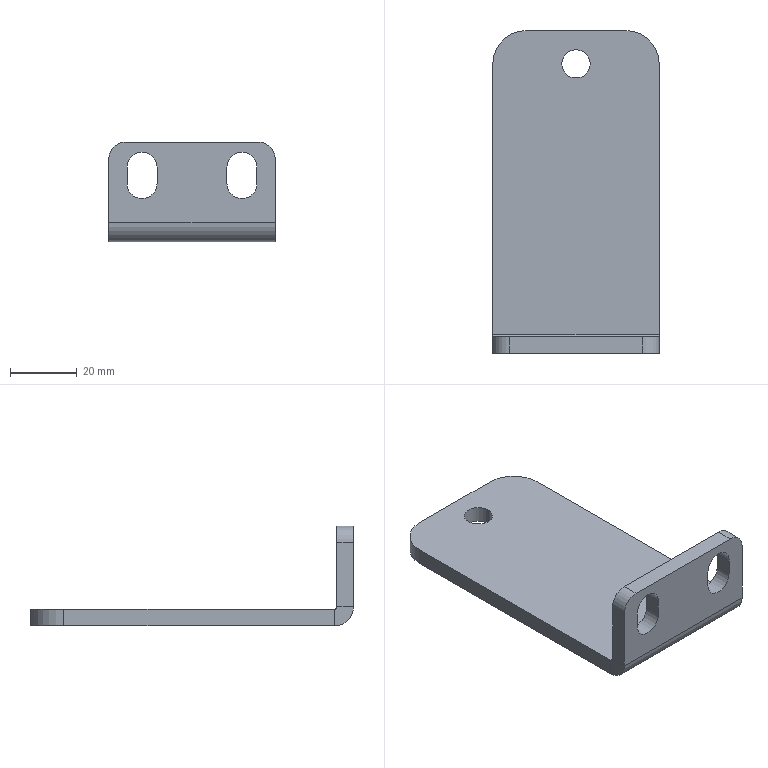Part | SolidWorks | features BaseBody 1 | 1 solid | 30 faces | box 50 x 97 x 30 mm | volume 28515 mm3 | plane 16 | cylinder 14 | commonest cylinder face diameters 9 x6 8.5 x2 10 x2 20 x2 1.473 x1 11.473 x1
STEP:
#1=CARTESIAN_POINT('',(-15.,-48.5,22.));
#2=VERTEX_POINT('',#1);
#3=CARTESIAN_POINT('',(-10.5,-48.5,17.5));
#4=VERTEX_POINT('',#3);
#5=CARTESIAN_POINT('',(-15.,-48.5,17.5));
#6=DIRECTION('',(0.,1.,0.));
#7=DIRECTION('',(0.,0.,1.));
#8=AXIS2_PLACEMENT_3D('',#5,#6,#7);
#9=CIRCLE('',#8,4.5);
#10=EDGE_CURVE('',#2,#4,#9,.T.);
#11=ORIENTED_EDGE('',*,*,#10,.F.);
#12=CARTESIAN_POINT('',(-15.,-43.5,22.));
#13=VERTEX_POINT('',#12);
#14=CARTESIAN_POINT('',(-15.,-53.5,22.));
#15=DIRECTION('',(0.,1.,0.));
#16=VECTOR('',#15,1000.);
#17=LINE('',#14,#16);
#18=EDGE_CURVE('',#2,#13,#17,.T.);
#19=ORIENTED_EDGE('',*,*,#18,.T.);
#20=CARTESIAN_POINT('',(-10.5,-43.5,17.5));
#21=VERTEX_POINT('',#20);
#22=CARTESIAN_POINT('',(-15.,-43.5,17.5));
#23=DIRECTION('',(0.,1.,0.));
#24=DIRECTION('',(0.,0.,1.));
#25=AXIS2_PLACEMENT_3D('',#22,#23,#24);
#26=CIRCLE('',#25,4.5);
#27=EDGE_CURVE('',#13,#21,#26,.T.);
#28=ORIENTED_EDGE('',*,*,#27,.T.);
#29=CARTESIAN_POINT('',(-10.5,-53.5,17.5));
#30=DIRECTION('',(0.,1.,0.));
#31=VECTOR('',#30,1000.);
#32=LINE('',#29,#31);
#33=EDGE_CURVE('',#4,#21,#32,.T.);
#34=ORIENTED_EDGE('',*,*,#33,.F.);
#35=EDGE_LOOP('',(#11,#19,#28,#34));
#36=FACE_OUTER_BOUND('',#35,.T.);
#37=CARTESIAN_POINT('',(-15.,-53.5,17.5));
#38=DIRECTION('',(0.,1.,0.));
#39=DIRECTION('',(0.,0.,1.));
#40=AXIS2_PLACEMENT_3D('',#37,#38,#39);
#41=CYLINDRICAL_SURFACE('',#40,4.5);
#42=ADVANCED_FACE('',(#36),#41,.F.);
#43=CARTESIAN_POINT('',(15.,-48.5,22.));
#44=VERTEX_POINT('',#43);
#45=CARTESIAN_POINT('',(19.5,-48.5,17.5));
#46=VERTEX_POINT('',#45);
#47=CARTESIAN_POINT('',(15.,-48.5,17.5));
#48=DIRECTION('',(0.,1.,0.));
#49=DIRECTION('',(0.,0.,1.));
#50=AXIS2_PLACEMENT_3D('',#47,#48,#49);
#51=CIRCLE('',#50,4.5);
#52=EDGE_CURVE('',#44,#46,#51,.T.);
#53=ORIENTED_EDGE('',*,*,#52,.F.);
#54=CARTESIAN_POINT('',(15.,-43.5,22.));
#55=VERTEX_POINT('',#54);
#56=CARTESIAN_POINT('',(15.,-53.5,22.));
#57=DIRECTION('',(0.,1.,0.));
#58=VECTOR('',#57,1000.);
#59=LINE('',#56,#58);
#60=EDGE_CURVE('',#44,#55,#59,.T.);
#61=ORIENTED_EDGE('',*,*,#60,.T.);
#62=CARTESIAN_POINT('',(19.5,-43.5,17.5));
#63=VERTEX_POINT('',#62);
#64=CARTESIAN_POINT('',(15.,-43.5,17.5));
#65=DIRECTION('',(0.,1.,0.));
#66=DIRECTION('',(0.,0.,1.));
#67=AXIS2_PLACEMENT_3D('',#64,#65,#66);
#68=CIRCLE('',#67,4.5);
#69=EDGE_CURVE('',#55,#63,#68,.T.);
#70=ORIENTED_EDGE('',*,*,#69,.T.);
#71=CARTESIAN_POINT('',(19.5,-53.5,17.5));
#72=DIRECTION('',(0.,1.,0.));
#73=VECTOR('',#72,1000.);
#74=LINE('',#71,#73);
#75=EDGE_CURVE('',#46,#63,#74,.T.);
#76=ORIENTED_EDGE('',*,*,#75,.F.);
#77=EDGE_LOOP('',(#53,#61,#70,#76));
#78=FACE_OUTER_BOUND('',#77,.T.);
#79=CARTESIAN_POINT('',(15.,-53.5,17.5));
#80=DIRECTION('',(0.,1.,0.));
#81=DIRECTION('',(0.,0.,1.));
#82=AXIS2_PLACEMENT_3D('',#79,#80,#81);
#83=CYLINDRICAL_SURFACE('',#82,4.5);
#84=ADVANCED_FACE('',(#78),#83,.F.);
#85=CARTESIAN_POINT('',(-4.25,38.5,-5.));
#86=VERTEX_POINT('',#85);
#87=CARTESIAN_POINT('',(4.25,38.5,-5.));
#88=VERTEX_POINT('',#87);
#89=CARTESIAN_POINT('',(0.,38.5,-5.));
#90=DIRECTION('',(0.,0.,1.));
#91=DIRECTION('',(1.,0.,0.));
#92=AXIS2_PLACEMENT_3D('',#89,#90,#91);
#93=CIRCLE('',#92,4.25);
#94=EDGE_CURVE('',#86,#88,#93,.T.);
#95=ORIENTED_EDGE('',*,*,#94,.F.);
#96=CARTESIAN_POINT('',(-4.25,38.5,0.));
#97=VERTEX_POINT('',#96);
#98=CARTESIAN_POINT('',(-4.25,38.5,-5.));
#99=DIRECTION('',(0.,0.,1.));
#100=VECTOR('',#99,1000.);
#101=LINE('',#98,#100);
#102=EDGE_CURVE('',#86,#97,#101,.T.);
#103=ORIENTED_EDGE('',*,*,#102,.T.);
#104=CARTESIAN_POINT('',(4.25,38.5,0.));
#105=VERTEX_POINT('',#104);
#106=CARTESIAN_POINT('',(0.,38.5,0.));
#107=DIRECTION('',(0.,0.,1.));
#108=DIRECTION('',(1.,0.,0.));
#109=AXIS2_PLACEMENT_3D('',#106,#107,#108);
#110=CIRCLE('',#109,4.25);
#111=EDGE_CURVE('',#97,#105,#110,.T.);
#112=ORIENTED_EDGE('',*,*,#111,.T.);
#113=CARTESIAN_POINT('',(4.25,38.5,-5.));
#114=DIRECTION('',(0.,0.,1.));
#115=VECTOR('',#114,1000.);
#116=LINE('',#113,#115);
#117=EDGE_CURVE('',#88,#105,#116,.T.);
#118=ORIENTED_EDGE('',*,*,#117,.F.);
#119=EDGE_LOOP('',(#95,#103,#112,#118));
#120=FACE_OUTER_BOUND('',#119,.T.);
#121=CARTESIAN_POINT('',(0.,38.5,-5.));
#122=DIRECTION('',(0.,0.,1.));
#123=DIRECTION('',(1.,0.,0.));
#124=AXIS2_PLACEMENT_3D('',#121,#122,#123);
#125=CYLINDRICAL_SURFACE('',#124,4.25);
#126=ADVANCED_FACE('',(#120),#125,.F.);
#127=CARTESIAN_POINT('',(25.,-42.763,0.));
#128=VERTEX_POINT('',#127);
#129=CARTESIAN_POINT('',(25.,38.5,0.));
#130=VERTEX_POINT('',#129);
#131=CARTESIAN_POINT('',(25.,38.5,0.));
#132=DIRECTION('',(0.,1.,0.));
#133=VECTOR('',#132,1000.);
#134=LINE('',#131,#133);
#135=EDGE_CURVE('',#128,#130,#134,.T.);
#136=ORIENTED_EDGE('',*,*,#135,.F.);
#137=CARTESIAN_POINT('',(25.,-42.763,-5.));
#138=VERTEX_POINT('',#137);
#139=CARTESIAN_POINT('',(25.,-42.763,0.));
#140=DIRECTION('',(0.,0.,-1.));
#141=VECTOR('',#140,1000.);
#142=LINE('',#139,#141);
#143=EDGE_CURVE('',#128,#138,#142,.T.);
#144=ORIENTED_EDGE('',*,*,#143,.T.);
#145=CARTESIAN_POINT('',(25.,38.5,-5.));
#146=VERTEX_POINT('',#145);
#147=CARTESIAN_POINT('',(25.,38.5,-5.));
#148=DIRECTION('',(0.,1.,0.));
#149=VECTOR('',#148,1000.);
#150=LINE('',#147,#149);
#151=EDGE_CURVE('',#138,#146,#150,.T.);
#152=ORIENTED_EDGE('',*,*,#151,.T.);
#153=CARTESIAN_POINT('',(25.,38.5,-5.));
#154=DIRECTION('',(0.,0.,1.));
#155=VECTOR('',#154,1000.);
#156=LINE('',#153,#155);
#157=EDGE_CURVE('',#146,#130,#156,.T.);
#158=ORIENTED_EDGE('',*,*,#157,.T.);
#159=EDGE_LOOP('',(#136,#144,#152,#158));
#160=FACE_OUTER_BOUND('',#159,.T.);
#161=CARTESIAN_POINT('',(25.,38.5,-5.));
#162=DIRECTION('',(1.,0.,0.));
#163=DIRECTION('',(0.,1.,0.));
#164=AXIS2_PLACEMENT_3D('',#161,#162,#163);
#165=PLANE('',#164);
#166=ADVANCED_FACE('',(#160),#165,.T.);
#167=CARTESIAN_POINT('',(0.,38.5,-5.));
#168=DIRECTION('',(0.,0.,1.));
#169=DIRECTION('',(1.,0.,0.));
#170=AXIS2_PLACEMENT_3D('',#167,#168,#169);
#171=CIRCLE('',#170,4.25);
#172=EDGE_CURVE('',#88,#86,#171,.T.);
#173=ORIENTED_EDGE('',*,*,#172,.T.);
#174=ORIENTED_EDGE('',*,*,#94,.T.);
#175=EDGE_LOOP('',(#173,#174));
#176=FACE_BOUND('',#175,.T.);
#177=CARTESIAN_POINT('',(-25.,-42.763,-5.));
#178=VERTEX_POINT('',#177);
#179=CARTESIAN_POINT('',(25.,-42.763,-5.));
#180=DIRECTION('',(-1.,0.,0.));
#181=VECTOR('',#180,1000.);
#182=LINE('',#179,#181);
#183=EDGE_CURVE('',#138,#178,#182,.T.);
#184=ORIENTED_EDGE('',*,*,#183,.T.);
#185=CARTESIAN_POINT('',(-25.,38.5,-5.));
#186=VERTEX_POINT('',#185);
#187=CARTESIAN_POINT('',(-25.,38.5,-5.));
#188=DIRECTION('',(0.,-1.,0.));
#189=VECTOR('',#188,1000.);
#190=LINE('',#187,#189);
#191=EDGE_CURVE('',#186,#178,#190,.T.);
#192=ORIENTED_EDGE('',*,*,#191,.F.);
#193=CARTESIAN_POINT('',(-15.,48.5,-5.));
#194=VERTEX_POINT('',#193);
#195=CARTESIAN_POINT('',(-15.,38.5,-5.));
#196=DIRECTION('',(0.,0.,1.));
#197=DIRECTION('',(1.,0.,0.));
#198=AXIS2_PLACEMENT_3D('',#195,#196,#197);
#199=CIRCLE('',#198,10.);
#200=EDGE_CURVE('',#194,#186,#199,.T.);
#201=ORIENTED_EDGE('',*,*,#200,.F.);
#202=CARTESIAN_POINT('',(15.,48.5,-5.));
#203=VERTEX_POINT('',#202);
#204=CARTESIAN_POINT('',(-15.,48.5,-5.));
#205=DIRECTION('',(-1.,0.,0.));
#206=VECTOR('',#205,1000.);
#207=LINE('',#204,#206);
#208=EDGE_CURVE('',#203,#194,#207,.T.);
#209=ORIENTED_EDGE('',*,*,#208,.F.);
#210=CARTESIAN_POINT('',(15.,38.5,-5.));
#211=DIRECTION('',(0.,0.,1.));
#212=DIRECTION('',(-1.,0.,0.));
#213=AXIS2_PLACEMENT_3D('',#210,#211,#212);
#214=CIRCLE('',#213,10.);
#215=EDGE_CURVE('',#146,#203,#214,.T.);
#216=ORIENTED_EDGE('',*,*,#215,.F.);
#217=ORIENTED_EDGE('',*,*,#151,.F.);
#218=EDGE_LOOP('',(#184,#192,#201,#209,#216,#217));
#219=FACE_OUTER_BOUND('',#218,.T.);
#220=CARTESIAN_POINT('',(-15.,38.5,-5.));
#221=DIRECTION('',(0.,0.,1.));
#222=DIRECTION('',(1.,0.,0.));
#223=AXIS2_PLACEMENT_3D('',#220,#221,#222);
#224=PLANE('',#223);
#225=ADVANCED_FACE('',(#176,#219),#224,.F.);
#226=CARTESIAN_POINT('',(0.,38.5,0.));
#227=DIRECTION('',(0.,0.,1.));
#228=DIRECTION('',(1.,0.,0.));
#229=AXIS2_PLACEMENT_3D('',#226,#227,#228);
#230=CIRCLE('',#229,4.25);
#231=EDGE_CURVE('',#105,#97,#230,.T.);
#232=ORIENTED_EDGE('',*,*,#231,.F.);
#233=ORIENTED_EDGE('',*,*,#111,.F.);
#234=EDGE_LOOP('',(#232,#233));
#235=FACE_BOUND('',#234,.T.);
#236=CARTESIAN_POINT('',(-25.,38.5,0.));
#237=VERTEX_POINT('',#236);
#238=CARTESIAN_POINT('',(-25.,-42.763,0.));
#239=VERTEX_POINT('',#238);
#240=CARTESIAN_POINT('',(-25.,38.5,0.));
#241=DIRECTION('',(0.,-1.,0.));
#242=VECTOR('',#241,1000.);
#243=LINE('',#240,#242);
#244=EDGE_CURVE('',#237,#239,#243,.T.);
#245=ORIENTED_EDGE('',*,*,#244,.T.);
#246=CARTESIAN_POINT('',(25.,-42.763,0.));
#247=DIRECTION('',(-1.,0.,0.));
#248=VECTOR('',#247,1000.);
#249=LINE('',#246,#248);
#250=EDGE_CURVE('',#128,#239,#249,.T.);
#251=ORIENTED_EDGE('',*,*,#250,.F.);
#252=ORIENTED_EDGE('',*,*,#135,.T.);
#253=CARTESIAN_POINT('',(15.,48.5,0.));
#254=VERTEX_POINT('',#253);
#255=CARTESIAN_POINT('',(15.,38.5,0.));
#256=DIRECTION('',(0.,0.,1.));
#257=DIRECTION('',(-1.,0.,0.));
#258=AXIS2_PLACEMENT_3D('',#255,#256,#257);
#259=CIRCLE('',#258,10.);
#260=EDGE_CURVE('',#130,#254,#259,.T.);
#261=ORIENTED_EDGE('',*,*,#260,.T.);
#262=CARTESIAN_POINT('',(-15.,48.5,0.));
#263=VERTEX_POINT('',#262);
#264=CARTESIAN_POINT('',(-15.,48.5,0.));
#265=DIRECTION('',(-1.,0.,0.));
#266=VECTOR('',#265,1000.);
#267=LINE('',#264,#266);
#268=EDGE_CURVE('',#254,#263,#267,.T.);
#269=ORIENTED_EDGE('',*,*,#268,.T.);
#270=CARTESIAN_POINT('',(-15.,38.5,0.));
#271=DIRECTION('',(0.,0.,1.));
#272=DIRECTION('',(1.,0.,0.));
#273=AXIS2_PLACEMENT_3D('',#270,#271,#272);
#274=CIRCLE('',#273,10.);
#275=EDGE_CURVE('',#263,#237,#274,.T.);
#276=ORIENTED_EDGE('',*,*,#275,.T.);
#277=EDGE_LOOP('',(#245,#251,#252,#261,#269,#276));
#278=FACE_OUTER_BOUND('',#277,.T.);
#279=CARTESIAN_POINT('',(-15.,38.5,0.));
#280=DIRECTION('',(0.,0.,1.));
#281=DIRECTION('',(1.,0.,0.));
#282=AXIS2_PLACEMENT_3D('',#279,#280,#281);
#283=PLANE('',#282);
#284=ADVANCED_FACE('',(#235,#278),#283,.T.);
#285=CARTESIAN_POINT('',(-25.,-42.763,0.));
#286=DIRECTION('',(0.,0.,-1.));
#287=VECTOR('',#286,1000.);
#288=LINE('',#285,#287);
#289=EDGE_CURVE('',#239,#178,#288,.T.);
#290=ORIENTED_EDGE('',*,*,#289,.F.);
#291=ORIENTED_EDGE('',*,*,#244,.F.);
#292=CARTESIAN_POINT('',(-25.,38.5,-5.));
#293=DIRECTION('',(0.,0.,1.));
#294=VECTOR('',#293,1000.);
#295=LINE('',#292,#294);
#296=EDGE_CURVE('',#186,#237,#295,.T.);
#297=ORIENTED_EDGE('',*,*,#296,.F.);
#298=ORIENTED_EDGE('',*,*,#191,.T.);
#299=EDGE_LOOP('',(#290,#291,#297,#298));
#300=FACE_OUTER_BOUND('',#299,.T.);
#301=CARTESIAN_POINT('',(-25.,38.5,-5.));
#302=DIRECTION('',(-1.,0.,0.));
#303=DIRECTION('',(0.,-1.,0.));
#304=AXIS2_PLACEMENT_3D('',#301,#302,#303);
#305=PLANE('',#304);
#306=ADVANCED_FACE('',(#300),#305,.T.);
#307=ORIENTED_EDGE('',*,*,#275,.F.);
#308=CARTESIAN_POINT('',(-15.,48.5,-5.));
#309=DIRECTION('',(0.,0.,1.));
#310=VECTOR('',#309,1000.);
#311=LINE('',#308,#310);
#312=EDGE_CURVE('',#194,#263,#311,.T.);
#313=ORIENTED_EDGE('',*,*,#312,.F.);
#314=ORIENTED_EDGE('',*,*,#200,.T.);
#315=ORIENTED_EDGE('',*,*,#296,.T.);
#316=EDGE_LOOP('',(#307,#313,#314,#315));
#317=FACE_OUTER_BOUND('',#316,.T.);
#318=CARTESIAN_POINT('',(-15.,38.5,-5.));
#319=DIRECTION('',(0.,0.,1.));
#320=DIRECTION('',(1.,0.,0.));
#321=AXIS2_PLACEMENT_3D('',#318,#319,#320);
#322=CYLINDRICAL_SURFACE('',#321,10.);
#323=ADVANCED_FACE('',(#317),#322,.T.);
#324=ORIENTED_EDGE('',*,*,#268,.F.);
#325=CARTESIAN_POINT('',(15.,48.5,-5.));
#326=DIRECTION('',(0.,0.,1.));
#327=VECTOR('',#326,1000.);
#328=LINE('',#325,#327);
#329=EDGE_CURVE('',#203,#254,#328,.T.);
#330=ORIENTED_EDGE('',*,*,#329,.F.);
#331=ORIENTED_EDGE('',*,*,#208,.T.);
#332=ORIENTED_EDGE('',*,*,#312,.T.);
#333=EDGE_LOOP('',(#324,#330,#331,#332));
#334=FACE_OUTER_BOUND('',#333,.T.);
#335=CARTESIAN_POINT('',(-15.,48.5,-5.));
#336=DIRECTION('',(0.,1.,0.));
#337=DIRECTION('',(0.,0.,1.));
#338=AXIS2_PLACEMENT_3D('',#335,#336,#337);
#339=PLANE('',#338);
#340=ADVANCED_FACE('',(#334),#339,.T.);
#341=ORIENTED_EDGE('',*,*,#260,.F.);
#342=ORIENTED_EDGE('',*,*,#157,.F.);
#343=ORIENTED_EDGE('',*,*,#215,.T.);
#344=ORIENTED_EDGE('',*,*,#329,.T.);
#345=EDGE_LOOP('',(#341,#342,#343,#344));
#346=FACE_OUTER_BOUND('',#345,.T.);
#347=CARTESIAN_POINT('',(15.,38.5,-5.));
#348=DIRECTION('',(0.,0.,1.));
#349=DIRECTION('',(1.,0.,0.));
#350=AXIS2_PLACEMENT_3D('',#347,#348,#349);
#351=CYLINDRICAL_SURFACE('',#350,10.);
#352=ADVANCED_FACE('',(#346),#351,.T.);
#353=ORIENTED_EDGE('',*,*,#102,.F.);
#354=ORIENTED_EDGE('',*,*,#172,.F.);
#355=ORIENTED_EDGE('',*,*,#117,.T.);
#356=ORIENTED_EDGE('',*,*,#231,.T.);
#357=EDGE_LOOP('',(#353,#354,#355,#356));
#358=FACE_OUTER_BOUND('',#357,.T.);
#359=CARTESIAN_POINT('',(0.,38.5,-5.));
#360=DIRECTION('',(0.,0.,1.));
#361=DIRECTION('',(1.,0.,0.));
#362=AXIS2_PLACEMENT_3D('',#359,#360,#361);
#363=CYLINDRICAL_SURFACE('',#362,4.25);
#364=ADVANCED_FACE('',(#358),#363,.F.);
#365=CARTESIAN_POINT('',(-25.,-43.5,0.7366));
#366=VERTEX_POINT('',#365);
#367=CARTESIAN_POINT('',(-25.,-48.5,0.7366));
#368=VERTEX_POINT('',#367);
#369=CARTESIAN_POINT('',(-25.,-48.5,0.7366));
#370=DIRECTION('',(0.,-1.,0.));
#371=VECTOR('',#370,1000.);
#372=LINE('',#369,#371);
#373=EDGE_CURVE('',#366,#368,#372,.T.);
#374=ORIENTED_EDGE('',*,*,#373,.F.);
#375=CARTESIAN_POINT('',(-25.,-42.763,0.7366));
#376=DIRECTION('',(-1.,0.,0.));
#377=DIRECTION('',(0.,0.,-1.));
#378=AXIS2_PLACEMENT_3D('',#375,#376,#377);
#379=CIRCLE('',#378,0.7366);
#380=EDGE_CURVE('',#239,#366,#379,.T.);
#381=ORIENTED_EDGE('',*,*,#380,.F.);
#382=ORIENTED_EDGE('',*,*,#289,.T.);
#383=CARTESIAN_POINT('',(-25.,-42.763,0.7366));
#384=DIRECTION('',(-1.,0.,0.));
#385=DIRECTION('',(0.,0.,-1.));
#386=AXIS2_PLACEMENT_3D('',#383,#384,#385);
#387=CIRCLE('',#386,5.737);
#388=EDGE_CURVE('',#178,#368,#387,.T.);
#389=ORIENTED_EDGE('',*,*,#388,.T.);
#390=EDGE_LOOP('',(#374,#381,#382,#389));
#391=FACE_OUTER_BOUND('',#390,.T.);
#392=CARTESIAN_POINT('',(-25.,-42.763,0.7366));
#393=DIRECTION('',(-1.,0.,0.));
#394=DIRECTION('',(0.,0.,1.));
#395=AXIS2_PLACEMENT_3D('',#392,#393,#394);
#396=PLANE('',#395);
#397=ADVANCED_FACE('',(#391),#396,.T.);
#398=CARTESIAN_POINT('',(25.,-43.5,0.7366));
#399=VERTEX_POINT('',#398);
#400=CARTESIAN_POINT('',(25.,-42.763,0.7366));
#401=DIRECTION('',(1.,0.,0.));
#402=DIRECTION('',(0.,0.,-1.));
#403=AXIS2_PLACEMENT_3D('',#400,#401,#402);
#404=CIRCLE('',#403,0.7366);
#405=EDGE_CURVE('',#399,#128,#404,.T.);
#406=ORIENTED_EDGE('',*,*,#405,.F.);
#407=CARTESIAN_POINT('',(25.,-48.5,0.7366));
#408=VERTEX_POINT('',#407);
#409=CARTESIAN_POINT('',(25.,-43.5,0.7366));
#410=DIRECTION('',(0.,-1.,0.));
#411=VECTOR('',#410,1000.);
#412=LINE('',#409,#411);
#413=EDGE_CURVE('',#399,#408,#412,.T.);
#414=ORIENTED_EDGE('',*,*,#413,.T.);
#415=CARTESIAN_POINT('',(25.,-42.763,0.7366));
#416=DIRECTION('',(1.,0.,0.));
#417=DIRECTION('',(0.,0.,-1.));
#418=AXIS2_PLACEMENT_3D('',#415,#416,#417);
#419=CIRCLE('',#418,5.737);
#420=EDGE_CURVE('',#408,#138,#419,.T.);
#421=ORIENTED_EDGE('',*,*,#420,.T.);
#422=ORIENTED_EDGE('',*,*,#143,.F.);
#423=EDGE_LOOP('',(#406,#414,#421,#422));
#424=FACE_OUTER_BOUND('',#423,.T.);
#425=CARTESIAN_POINT('',(25.,-42.763,0.7366));
#426=DIRECTION('',(-1.,0.,0.));
#427=DIRECTION('',(0.,0.,1.));
#428=AXIS2_PLACEMENT_3D('',#425,#426,#427);
#429=PLANE('',#428);
#430=ADVANCED_FACE('',(#424),#429,.F.);
#431=ORIENTED_EDGE('',*,*,#183,.F.);
#432=ORIENTED_EDGE('',*,*,#420,.F.);
#433=CARTESIAN_POINT('',(-25.,-48.5,0.7366));
#434=DIRECTION('',(-1.,0.,0.));
#435=VECTOR('',#434,1000.);
#436=LINE('',#433,#435);
#437=EDGE_CURVE('',#408,#368,#436,.T.);
#438=ORIENTED_EDGE('',*,*,#437,.T.);
#439=ORIENTED_EDGE('',*,*,#388,.F.);
#440=EDGE_LOOP('',(#431,#432,#438,#439));
#441=FACE_OUTER_BOUND('',#440,.T.);
#442=CARTESIAN_POINT('',(25.,-42.763,0.7366));
#443=DIRECTION('',(1.,0.,0.));
#444=DIRECTION('',(0.,-1.,0.));
#445=AXIS2_PLACEMENT_3D('',#442,#443,#444);
#446=CYLINDRICAL_SURFACE('',#445,5.737);
#447=ADVANCED_FACE('',(#441),#446,.T.);
#448=ORIENTED_EDGE('',*,*,#250,.T.);
#449=ORIENTED_EDGE('',*,*,#380,.T.);
#450=CARTESIAN_POINT('',(-25.,-43.5,0.7366));
#451=DIRECTION('',(1.,0.,0.));
#452=VECTOR('',#451,1000.);
#453=LINE('',#450,#452);
#454=EDGE_CURVE('',#366,#399,#453,.T.);
#455=ORIENTED_EDGE('',*,*,#454,.T.);
#456=ORIENTED_EDGE('',*,*,#405,.T.);
#457=EDGE_LOOP('',(#448,#449,#455,#456));
#458=FACE_OUTER_BOUND('',#457,.T.);
#459=CARTESIAN_POINT('',(25.,-42.763,0.7366));
#460=DIRECTION('',(1.,0.,0.));
#461=DIRECTION('',(0.,-1.,0.));
#462=AXIS2_PLACEMENT_3D('',#459,#460,#461);
#463=CYLINDRICAL_SURFACE('',#462,0.7366);
#464=ADVANCED_FACE('',(#458),#463,.F.);
#465=CARTESIAN_POINT('',(-25.,-48.5,20.));
#466=VERTEX_POINT('',#465);
#467=CARTESIAN_POINT('',(-25.,-48.5,0.));
#468=DIRECTION('',(0.,0.,-1.));
#469=VECTOR('',#468,1000.);
#470=LINE('',#467,#469);
#471=EDGE_CURVE('',#466,#368,#470,.T.);
#472=ORIENTED_EDGE('',*,*,#471,.F.);
#473=CARTESIAN_POINT('',(-25.,-43.5,20.));
#474=VERTEX_POINT('',#473);
#475=CARTESIAN_POINT('',(-25.,-48.5,20.));
#476=DIRECTION('',(0.,1.,0.));
#477=VECTOR('',#476,1000.);
#478=LINE('',#475,#477);
#479=EDGE_CURVE('',#466,#474,#478,.T.);
#480=ORIENTED_EDGE('',*,*,#479,.T.);
#481=CARTESIAN_POINT('',(-25.,-43.5,0.));
#482=DIRECTION('',(0.,0.,-1.));
#483=VECTOR('',#482,1000.);
#484=LINE('',#481,#483);
#485=EDGE_CURVE('',#474,#366,#484,.T.);
#486=ORIENTED_EDGE('',*,*,#485,.T.);
#487=ORIENTED_EDGE('',*,*,#373,.T.);
#488=EDGE_LOOP('',(#472,#480,#486,#487));
#489=FACE_OUTER_BOUND('',#488,.T.);
#490=CARTESIAN_POINT('',(-25.,-48.5,0.));
#491=DIRECTION('',(1.,0.,0.));
#492=DIRECTION('',(0.,0.,-1.));
#493=AXIS2_PLACEMENT_3D('',#490,#491,#492);
#494=PLANE('',#493);
#495=ADVANCED_FACE('',(#489),#494,.F.);
#496=CARTESIAN_POINT('',(25.,-43.5,20.));
#497=VERTEX_POINT('',#496);
#498=CARTESIAN_POINT('',(25.,-43.5,25.));
#499=DIRECTION('',(0.,0.,1.));
#500=VECTOR('',#499,1000.);
#501=LINE('',#498,#500);
#502=EDGE_CURVE('',#399,#497,#501,.T.);
#503=ORIENTED_EDGE('',*,*,#502,.T.);
#504=CARTESIAN_POINT('',(25.,-48.5,20.));
#505=VERTEX_POINT('',#504);
#506=CARTESIAN_POINT('',(25.,-48.5,20.));
#507=DIRECTION('',(0.,-1.,0.));
#508=VECTOR('',#507,1000.);
#509=LINE('',#506,#508);
#510=EDGE_CURVE('',#497,#505,#509,.T.);
#511=ORIENTED_EDGE('',*,*,#510,.T.);
#512=CARTESIAN_POINT('',(25.,-48.5,0.));
#513=DIRECTION('',(0.,0.,1.));
#514=VECTOR('',#513,1000.);
#515=LINE('',#512,#514);
#516=EDGE_CURVE('',#408,#505,#515,.T.);
#517=ORIENTED_EDGE('',*,*,#516,.F.);
#518=ORIENTED_EDGE('',*,*,#413,.F.);
#519=EDGE_LOOP('',(#503,#511,#517,#518));
#520=FACE_OUTER_BOUND('',#519,.T.);
#521=CARTESIAN_POINT('',(25.,-48.5,25.));
#522=DIRECTION('',(-1.,0.,0.));
#523=DIRECTION('',(0.,0.,1.));
#524=AXIS2_PLACEMENT_3D('',#521,#522,#523);
#525=PLANE('',#524);
#526=ADVANCED_FACE('',(#520),#525,.F.);
#527=CARTESIAN_POINT('',(-10.5,-48.5,12.5));
#528=VERTEX_POINT('',#527);
#529=CARTESIAN_POINT('',(-10.5,-48.5,0.));
#530=DIRECTION('',(0.,0.,-1.));
#531=VECTOR('',#530,1000.);
#532=LINE('',#529,#531);
#533=EDGE_CURVE('',#4,#528,#532,.T.);
#534=ORIENTED_EDGE('',*,*,#533,.T.);
#535=CARTESIAN_POINT('',(-19.5,-48.5,12.5));
#536=VERTEX_POINT('',#535);
#537=CARTESIAN_POINT('',(-15.,-48.5,12.5));
#538=DIRECTION('',(0.,1.,0.));
#539=DIRECTION('',(0.,0.,1.));
#540=AXIS2_PLACEMENT_3D('',#537,#538,#539);
#541=CIRCLE('',#540,4.5);
#542=EDGE_CURVE('',#528,#536,#541,.T.);
#543=ORIENTED_EDGE('',*,*,#542,.T.);
#544=CARTESIAN_POINT('',(-19.5,-48.5,17.5));
#545=VERTEX_POINT('',#544);
#546=CARTESIAN_POINT('',(-19.5,-48.5,0.));
#547=DIRECTION('',(0.,0.,1.));
#548=VECTOR('',#547,1000.);
#549=LINE('',#546,#548);
#550=EDGE_CURVE('',#536,#545,#549,.T.);
#551=ORIENTED_EDGE('',*,*,#550,.T.);
#552=CARTESIAN_POINT('',(-15.,-48.5,17.5));
#553=DIRECTION('',(0.,1.,0.));
#554=DIRECTION('',(0.,0.,1.));
#555=AXIS2_PLACEMENT_3D('',#552,#553,#554);
#556=CIRCLE('',#555,4.5);
#557=EDGE_CURVE('',#545,#2,#556,.T.);
#558=ORIENTED_EDGE('',*,*,#557,.T.);
#559=ORIENTED_EDGE('',*,*,#10,.T.);
#560=EDGE_LOOP('',(#534,#543,#551,#558,#559));
#561=FACE_BOUND('',#560,.T.);
#562=CARTESIAN_POINT('',(19.5,-48.5,12.5));
#563=VERTEX_POINT('',#562);
#564=CARTESIAN_POINT('',(19.5,-48.5,0.));
#565=DIRECTION('',(0.,0.,-1.));
#566=VECTOR('',#565,1000.);
#567=LINE('',#564,#566);
#568=EDGE_CURVE('',#46,#563,#567,.T.);
#569=ORIENTED_EDGE('',*,*,#568,.T.);
#570=CARTESIAN_POINT('',(10.5,-48.5,12.5));
#571=VERTEX_POINT('',#570);
#572=CARTESIAN_POINT('',(15.,-48.5,12.5));
#573=DIRECTION('',(0.,1.,0.));
#574=DIRECTION('',(0.,0.,1.));
#575=AXIS2_PLACEMENT_3D('',#572,#573,#574);
#576=CIRCLE('',#575,4.5);
#577=EDGE_CURVE('',#563,#571,#576,.T.);
#578=ORIENTED_EDGE('',*,*,#577,.T.);
#579=CARTESIAN_POINT('',(10.5,-48.5,17.5));
#580=VERTEX_POINT('',#579);
#581=CARTESIAN_POINT('',(10.5,-48.5,0.));
#582=DIRECTION('',(0.,0.,1.));
#583=VECTOR('',#582,1000.);
#584=LINE('',#581,#583);
#585=EDGE_CURVE('',#571,#580,#584,.T.);
#586=ORIENTED_EDGE('',*,*,#585,.T.);
#587=CARTESIAN_POINT('',(15.,-48.5,17.5));
#588=DIRECTION('',(0.,1.,0.));
#589=DIRECTION('',(0.,0.,1.));
#590=AXIS2_PLACEMENT_3D('',#587,#588,#589);
#591=CIRCLE('',#590,4.5);
#592=EDGE_CURVE('',#580,#44,#591,.T.);
#593=ORIENTED_EDGE('',*,*,#592,.T.);
#594=ORIENTED_EDGE('',*,*,#52,.T.);
#595=EDGE_LOOP('',(#569,#578,#586,#593,#594));
#596=FACE_BOUND('',#595,.T.);
#597=CARTESIAN_POINT('',(20.,-48.5,25.));
#598=VERTEX_POINT('',#597);
#599=CARTESIAN_POINT('',(-20.,-48.5,25.));
#600=VERTEX_POINT('',#599);
#601=CARTESIAN_POINT('',(0.,-48.5,25.));
#602=DIRECTION('',(-1.,0.,0.));
#603=VECTOR('',#602,1000.);
#604=LINE('',#601,#603);
#605=EDGE_CURVE('',#598,#600,#604,.T.);
#606=ORIENTED_EDGE('',*,*,#605,.T.);
#607=CARTESIAN_POINT('',(-20.,-48.5,20.));
#608=DIRECTION('',(0.,-1.,0.));
#609=DIRECTION('',(0.,0.,1.));
#610=AXIS2_PLACEMENT_3D('',#607,#608,#609);
#611=CIRCLE('',#610,5.);
#612=EDGE_CURVE('',#600,#466,#611,.T.);
#613=ORIENTED_EDGE('',*,*,#612,.T.);
#614=ORIENTED_EDGE('',*,*,#471,.T.);
#615=ORIENTED_EDGE('',*,*,#437,.F.);
#616=ORIENTED_EDGE('',*,*,#516,.T.);
#617=CARTESIAN_POINT('',(20.,-48.5,20.));
#618=DIRECTION('',(0.,-1.,0.));
#619=DIRECTION('',(0.,0.,1.));
#620=AXIS2_PLACEMENT_3D('',#617,#618,#619);
#621=CIRCLE('',#620,5.);
#622=EDGE_CURVE('',#505,#598,#621,.T.);
#623=ORIENTED_EDGE('',*,*,#622,.T.);
#624=EDGE_LOOP('',(#606,#613,#614,#615,#616,#623));
#625=FACE_OUTER_BOUND('',#624,.T.);
#626=CARTESIAN_POINT('',(0.,-48.5,0.));
#627=DIRECTION('',(0.,1.,0.));
#628=DIRECTION('',(0.,0.,1.));
#629=AXIS2_PLACEMENT_3D('',#626,#627,#628);
#630=PLANE('',#629);
#631=ADVANCED_FACE('',(#561,#596,#625),#630,.F.);
#632=CARTESIAN_POINT('',(-10.5,-43.5,12.5));
#633=VERTEX_POINT('',#632);
#634=CARTESIAN_POINT('',(-19.5,-43.5,12.5));
#635=VERTEX_POINT('',#634);
#636=CARTESIAN_POINT('',(-15.,-43.5,12.5));
#637=DIRECTION('',(0.,1.,0.));
#638=DIRECTION('',(0.,0.,1.));
#639=AXIS2_PLACEMENT_3D('',#636,#637,#638);
#640=CIRCLE('',#639,4.5);
#641=EDGE_CURVE('',#633,#635,#640,.T.);
#642=ORIENTED_EDGE('',*,*,#641,.F.);
#643=CARTESIAN_POINT('',(-10.5,-43.5,12.5));
#644=DIRECTION('',(0.,0.,-1.));
#645=VECTOR('',#644,1000.);
#646=LINE('',#643,#645);
#647=EDGE_CURVE('',#21,#633,#646,.T.);
#648=ORIENTED_EDGE('',*,*,#647,.F.);
#649=ORIENTED_EDGE('',*,*,#27,.F.);
#650=CARTESIAN_POINT('',(-19.5,-43.5,17.5));
#651=VERTEX_POINT('',#650);
#652=CARTESIAN_POINT('',(-15.,-43.5,17.5));
#653=DIRECTION('',(0.,1.,0.));
#654=DIRECTION('',(0.,0.,1.));
#655=AXIS2_PLACEMENT_3D('',#652,#653,#654);
#656=CIRCLE('',#655,4.5);
#657=EDGE_CURVE('',#651,#13,#656,.T.);
#658=ORIENTED_EDGE('',*,*,#657,.F.);
#659=CARTESIAN_POINT('',(-19.5,-43.5,12.5));
#660=DIRECTION('',(0.,0.,1.));
#661=VECTOR('',#660,1000.);
#662=LINE('',#659,#661);
#663=EDGE_CURVE('',#635,#651,#662,.T.);
#664=ORIENTED_EDGE('',*,*,#663,.F.);
#665=EDGE_LOOP('',(#642,#648,#649,#658,#664));
#666=FACE_BOUND('',#665,.T.);
#667=CARTESIAN_POINT('',(19.5,-43.5,12.5));
#668=VERTEX_POINT('',#667);
#669=CARTESIAN_POINT('',(10.5,-43.5,12.5));
#670=VERTEX_POINT('',#669);
#671=CARTESIAN_POINT('',(15.,-43.5,12.5));
#672=DIRECTION('',(0.,1.,0.));
#673=DIRECTION('',(0.,0.,1.));
#674=AXIS2_PLACEMENT_3D('',#671,#672,#673);
#675=CIRCLE('',#674,4.5);
#676=EDGE_CURVE('',#668,#670,#675,.T.);
#677=ORIENTED_EDGE('',*,*,#676,.F.);
#678=CARTESIAN_POINT('',(19.5,-43.5,12.5));
#679=DIRECTION('',(0.,0.,-1.));
#680=VECTOR('',#679,1000.);
#681=LINE('',#678,#680);
#682=EDGE_CURVE('',#63,#668,#681,.T.);
#683=ORIENTED_EDGE('',*,*,#682,.F.);
#684=ORIENTED_EDGE('',*,*,#69,.F.);
#685=CARTESIAN_POINT('',(10.5,-43.5,17.5));
#686=VERTEX_POINT('',#685);
#687=CARTESIAN_POINT('',(15.,-43.5,17.5));
#688=DIRECTION('',(0.,1.,0.));
#689=DIRECTION('',(0.,0.,1.));
#690=AXIS2_PLACEMENT_3D('',#687,#688,#689);
#691=CIRCLE('',#690,4.5);
#692=EDGE_CURVE('',#686,#55,#691,.T.);
#693=ORIENTED_EDGE('',*,*,#692,.F.);
#694=CARTESIAN_POINT('',(10.5,-43.5,12.5));
#695=DIRECTION('',(0.,0.,1.));
#696=VECTOR('',#695,1000.);
#697=LINE('',#694,#696);
#698=EDGE_CURVE('',#670,#686,#697,.T.);
#699=ORIENTED_EDGE('',*,*,#698,.F.);
#700=EDGE_LOOP('',(#677,#683,#684,#693,#699));
#701=FACE_BOUND('',#700,.T.);
#702=ORIENTED_EDGE('',*,*,#485,.F.);
#703=CARTESIAN_POINT('',(-20.,-43.5,25.));
#704=VERTEX_POINT('',#703);
#705=CARTESIAN_POINT('',(-20.,-43.5,20.));
#706=DIRECTION('',(0.,1.,0.));
#707=DIRECTION('',(0.,0.,1.));
#708=AXIS2_PLACEMENT_3D('',#705,#706,#707);
#709=CIRCLE('',#708,5.);
#710=EDGE_CURVE('',#474,#704,#709,.T.);
#711=ORIENTED_EDGE('',*,*,#710,.T.);
#712=CARTESIAN_POINT('',(20.,-43.5,25.));
#713=VERTEX_POINT('',#712);
#714=CARTESIAN_POINT('',(-25.,-43.5,25.));
#715=DIRECTION('',(-1.,0.,0.));
#716=VECTOR('',#715,1000.);
#717=LINE('',#714,#716);
#718=EDGE_CURVE('',#713,#704,#717,.T.);
#719=ORIENTED_EDGE('',*,*,#718,.F.);
#720=CARTESIAN_POINT('',(20.,-43.5,20.));
#721=DIRECTION('',(0.,1.,0.));
#722=DIRECTION('',(0.,0.,1.));
#723=AXIS2_PLACEMENT_3D('',#720,#721,#722);
#724=CIRCLE('',#723,5.);
#725=EDGE_CURVE('',#713,#497,#724,.T.);
#726=ORIENTED_EDGE('',*,*,#725,.T.);
#727=ORIENTED_EDGE('',*,*,#502,.F.);
#728=ORIENTED_EDGE('',*,*,#454,.F.);
#729=EDGE_LOOP('',(#702,#711,#719,#726,#727,#728));
#730=FACE_OUTER_BOUND('',#729,.T.);
#731=CARTESIAN_POINT('',(0.,-43.5,0.));
#732=DIRECTION('',(0.,1.,0.));
#733=DIRECTION('',(0.,0.,1.));
#734=AXIS2_PLACEMENT_3D('',#731,#732,#733);
#735=PLANE('',#734);
#736=ADVANCED_FACE('',(#666,#701,#730),#735,.T.);
#737=ORIENTED_EDGE('',*,*,#718,.T.);
#738=CARTESIAN_POINT('',(-20.,-48.5,25.));
#739=DIRECTION('',(0.,-1.,0.));
#740=VECTOR('',#739,1000.);
#741=LINE('',#738,#740);
#742=EDGE_CURVE('',#704,#600,#741,.T.);
#743=ORIENTED_EDGE('',*,*,#742,.T.);
#744=ORIENTED_EDGE('',*,*,#605,.F.);
#745=CARTESIAN_POINT('',(20.,-48.5,25.));
#746=DIRECTION('',(0.,1.,0.));
#747=VECTOR('',#746,1000.);
#748=LINE('',#745,#747);
#749=EDGE_CURVE('',#598,#713,#748,.T.);
#750=ORIENTED_EDGE('',*,*,#749,.T.);
#751=EDGE_LOOP('',(#737,#743,#744,#750));
#752=FACE_OUTER_BOUND('',#751,.T.);
#753=CARTESIAN_POINT('',(-25.,-48.5,25.));
#754=DIRECTION('',(0.,0.,-1.));
#755=DIRECTION('',(0.,1.,0.));
#756=AXIS2_PLACEMENT_3D('',#753,#754,#755);
#757=PLANE('',#756);
#758=ADVANCED_FACE('',(#752),#757,.F.);
#759=ORIENTED_EDGE('',*,*,#612,.F.);
#760=ORIENTED_EDGE('',*,*,#742,.F.);
#761=ORIENTED_EDGE('',*,*,#710,.F.);
#762=ORIENTED_EDGE('',*,*,#479,.F.);
#763=EDGE_LOOP('',(#759,#760,#761,#762));
#764=FACE_OUTER_BOUND('',#763,.T.);
#765=CARTESIAN_POINT('',(-20.,-48.5,20.));
#766=DIRECTION('',(0.,1.,0.));
#767=DIRECTION('',(0.,0.,1.));
#768=AXIS2_PLACEMENT_3D('',#765,#766,#767);
#769=CYLINDRICAL_SURFACE('',#768,5.);
#770=ADVANCED_FACE('',(#764),#769,.T.);
#771=ORIENTED_EDGE('',*,*,#622,.F.);
#772=ORIENTED_EDGE('',*,*,#510,.F.);
#773=ORIENTED_EDGE('',*,*,#725,.F.);
#774=ORIENTED_EDGE('',*,*,#749,.F.);
#775=EDGE_LOOP('',(#771,#772,#773,#774));
#776=FACE_OUTER_BOUND('',#775,.T.);
#777=CARTESIAN_POINT('',(20.,-48.5,20.));
#778=DIRECTION('',(0.,1.,0.));
#779=DIRECTION('',(0.,0.,1.));
#780=AXIS2_PLACEMENT_3D('',#777,#778,#779);
#781=CYLINDRICAL_SURFACE('',#780,5.);
#782=ADVANCED_FACE('',(#776),#781,.T.);
#783=CARTESIAN_POINT('',(19.5,-53.5,12.5));
#784=DIRECTION('',(0.,1.,0.));
#785=VECTOR('',#784,1000.);
#786=LINE('',#783,#785);
#787=EDGE_CURVE('',#563,#668,#786,.T.);
#788=ORIENTED_EDGE('',*,*,#787,.T.);
#789=ORIENTED_EDGE('',*,*,#676,.T.);
#790=CARTESIAN_POINT('',(10.5,-53.5,12.5));
#791=DIRECTION('',(0.,1.,0.));
#792=VECTOR('',#791,1000.);
#793=LINE('',#790,#792);
#794=EDGE_CURVE('',#571,#670,#793,.T.);
#795=ORIENTED_EDGE('',*,*,#794,.F.);
#796=ORIENTED_EDGE('',*,*,#577,.F.);
#797=EDGE_LOOP('',(#788,#789,#795,#796));
#798=FACE_OUTER_BOUND('',#797,.T.);
#799=CARTESIAN_POINT('',(15.,-53.5,12.5));
#800=DIRECTION('',(0.,1.,0.));
#801=DIRECTION('',(0.,0.,1.));
#802=AXIS2_PLACEMENT_3D('',#799,#800,#801);
#803=CYLINDRICAL_SURFACE('',#802,4.5);
#804=ADVANCED_FACE('',(#798),#803,.F.);
#805=ORIENTED_EDGE('',*,*,#75,.T.);
#806=ORIENTED_EDGE('',*,*,#682,.T.);
#807=ORIENTED_EDGE('',*,*,#787,.F.);
#808=ORIENTED_EDGE('',*,*,#568,.F.);
#809=EDGE_LOOP('',(#805,#806,#807,#808));
#810=FACE_OUTER_BOUND('',#809,.T.);
#811=CARTESIAN_POINT('',(19.5,-53.5,12.5));
#812=DIRECTION('',(1.,0.,0.));
#813=DIRECTION('',(0.,0.,-1.));
#814=AXIS2_PLACEMENT_3D('',#811,#812,#813);
#815=PLANE('',#814);
#816=ADVANCED_FACE('',(#810),#815,.F.);
#817=ORIENTED_EDGE('',*,*,#60,.F.);
#818=ORIENTED_EDGE('',*,*,#592,.F.);
#819=CARTESIAN_POINT('',(10.5,-53.5,17.5));
#820=DIRECTION('',(0.,1.,0.));
#821=VECTOR('',#820,1000.);
#822=LINE('',#819,#821);
#823=EDGE_CURVE('',#580,#686,#822,.T.);
#824=ORIENTED_EDGE('',*,*,#823,.T.);
#825=ORIENTED_EDGE('',*,*,#692,.T.);
#826=EDGE_LOOP('',(#817,#818,#824,#825));
#827=FACE_OUTER_BOUND('',#826,.T.);
#828=CARTESIAN_POINT('',(15.,-53.5,17.5));
#829=DIRECTION('',(0.,1.,0.));
#830=DIRECTION('',(0.,0.,1.));
#831=AXIS2_PLACEMENT_3D('',#828,#829,#830);
#832=CYLINDRICAL_SURFACE('',#831,4.5);
#833=ADVANCED_FACE('',(#827),#832,.F.);
#834=ORIENTED_EDGE('',*,*,#794,.T.);
#835=ORIENTED_EDGE('',*,*,#698,.T.);
#836=ORIENTED_EDGE('',*,*,#823,.F.);
#837=ORIENTED_EDGE('',*,*,#585,.F.);
#838=EDGE_LOOP('',(#834,#835,#836,#837));
#839=FACE_OUTER_BOUND('',#838,.T.);
#840=CARTESIAN_POINT('',(10.5,-53.5,12.5));
#841=DIRECTION('',(-1.,0.,0.));
#842=DIRECTION('',(0.,0.,1.));
#843=AXIS2_PLACEMENT_3D('',#840,#841,#842);
#844=PLANE('',#843);
#845=ADVANCED_FACE('',(#839),#844,.F.);
#846=CARTESIAN_POINT('',(-10.5,-53.5,12.5));
#847=DIRECTION('',(0.,1.,0.));
#848=VECTOR('',#847,1000.);
#849=LINE('',#846,#848);
#850=EDGE_CURVE('',#528,#633,#849,.T.);
#851=ORIENTED_EDGE('',*,*,#850,.T.);
#852=ORIENTED_EDGE('',*,*,#641,.T.);
#853=CARTESIAN_POINT('',(-19.5,-53.5,12.5));
#854=DIRECTION('',(0.,1.,0.));
#855=VECTOR('',#854,1000.);
#856=LINE('',#853,#855);
#857=EDGE_CURVE('',#536,#635,#856,.T.);
#858=ORIENTED_EDGE('',*,*,#857,.F.);
#859=ORIENTED_EDGE('',*,*,#542,.F.);
#860=EDGE_LOOP('',(#851,#852,#858,#859));
#861=FACE_OUTER_BOUND('',#860,.T.);
#862=CARTESIAN_POINT('',(-15.,-53.5,12.5));
#863=DIRECTION('',(0.,1.,0.));
#864=DIRECTION('',(0.,0.,1.));
#865=AXIS2_PLACEMENT_3D('',#862,#863,#864);
#866=CYLINDRICAL_SURFACE('',#865,4.5);
#867=ADVANCED_FACE('',(#861),#866,.F.);
#868=ORIENTED_EDGE('',*,*,#33,.T.);
#869=ORIENTED_EDGE('',*,*,#647,.T.);
#870=ORIENTED_EDGE('',*,*,#850,.F.);
#871=ORIENTED_EDGE('',*,*,#533,.F.);
#872=EDGE_LOOP('',(#868,#869,#870,#871));
#873=FACE_OUTER_BOUND('',#872,.T.);
#874=CARTESIAN_POINT('',(-10.5,-53.5,12.5));
#875=DIRECTION('',(1.,0.,0.));
#876=DIRECTION('',(0.,0.,-1.));
#877=AXIS2_PLACEMENT_3D('',#874,#875,#876);
#878=PLANE('',#877);
#879=ADVANCED_FACE('',(#873),#878,.F.);
#880=ORIENTED_EDGE('',*,*,#18,.F.);
#881=ORIENTED_EDGE('',*,*,#557,.F.);
#882=CARTESIAN_POINT('',(-19.5,-53.5,17.5));
#883=DIRECTION('',(0.,1.,0.));
#884=VECTOR('',#883,1000.);
#885=LINE('',#882,#884);
#886=EDGE_CURVE('',#545,#651,#885,.T.);
#887=ORIENTED_EDGE('',*,*,#886,.T.);
#888=ORIENTED_EDGE('',*,*,#657,.T.);
#889=EDGE_LOOP('',(#880,#881,#887,#888));
#890=FACE_OUTER_BOUND('',#889,.T.);
#891=CARTESIAN_POINT('',(-15.,-53.5,17.5));
#892=DIRECTION('',(0.,1.,0.));
#893=DIRECTION('',(0.,0.,1.));
#894=AXIS2_PLACEMENT_3D('',#891,#892,#893);
#895=CYLINDRICAL_SURFACE('',#894,4.5);
#896=ADVANCED_FACE('',(#890),#895,.F.);
#897=ORIENTED_EDGE('',*,*,#857,.T.);
#898=ORIENTED_EDGE('',*,*,#663,.T.);
#899=ORIENTED_EDGE('',*,*,#886,.F.);
#900=ORIENTED_EDGE('',*,*,#550,.F.);
#901=EDGE_LOOP('',(#897,#898,#899,#900));
#902=FACE_OUTER_BOUND('',#901,.T.);
#903=CARTESIAN_POINT('',(-19.5,-53.5,12.5));
#904=DIRECTION('',(-1.,0.,0.));
#905=DIRECTION('',(0.,0.,1.));
#906=AXIS2_PLACEMENT_3D('',#903,#904,#905);
#907=PLANE('',#906);
#908=ADVANCED_FACE('',(#902),#907,.F.);
#909=CLOSED_SHELL('',(#42,#84,#126,#166,#225,#284,#306,#323,#340,#352,#364,#397,#430,#447,#464,#495,#526,#631,#736,#758,#770,#782,#804,#816,#833,#845,#867,#879,#896,#908));
#910=MANIFOLD_SOLID_BREP('',#909);
#911=CARTESIAN_POINT('',(0.,0.,0.));
#912=DIRECTION('',(0.,0.,1.));
#913=DIRECTION('',(1.,0.,0.));
#914=AXIS2_PLACEMENT_3D('',#911,#912,#913);
#915=(LENGTH_UNIT()NAMED_UNIT(*)SI_UNIT(.MILLI.,.METRE.));
#916=UNCERTAINTY_MEASURE_WITH_UNIT(LENGTH_MEASURE(0.00001),#915,'','');
#917=(NAMED_UNIT(*)PLANE_ANGLE_UNIT()SI_UNIT($,.RADIAN.));
#918=(NAMED_UNIT(*)SI_UNIT($,.STERADIAN.)SOLID_ANGLE_UNIT());
#919=(GEOMETRIC_REPRESENTATION_CONTEXT(3)GLOBAL_UNCERTAINTY_ASSIGNED_CONTEXT((#916))GLOBAL_UNIT_ASSIGNED_CONTEXT((#915,#917,#918))REPRESENTATION_CONTEXT('',''));
#920=ADVANCED_BREP_SHAPE_REPRESENTATION('',(#910,#914),#919);